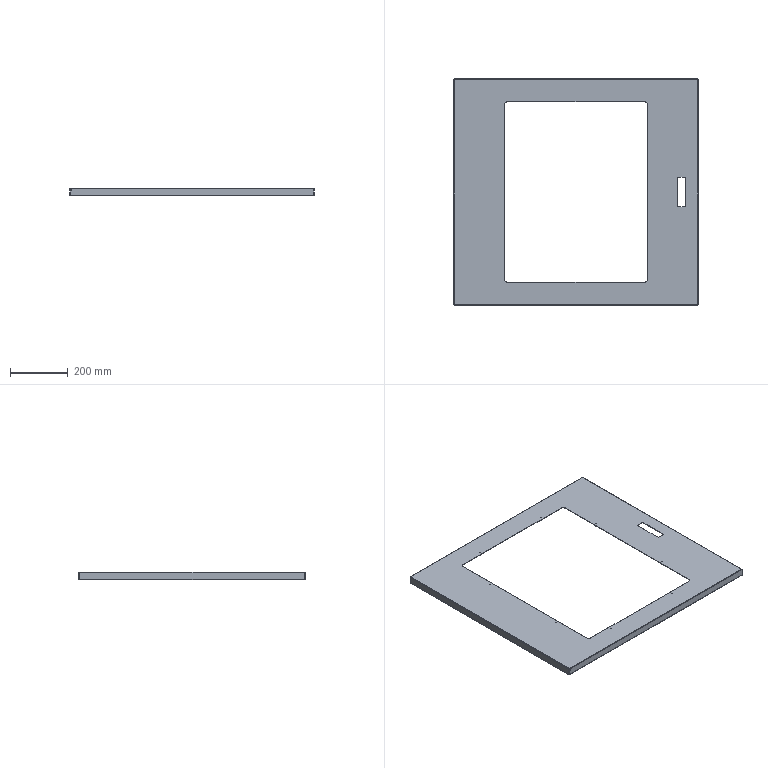Part | SolidWorks | features ICE 4, EdgeFlange 2, MirrorPattern 2, Fillet 1, FlatPattern 1, HoleWzd 1, SMBaseFlange 1, SheetMetal 1 | 1 solid | 110 faces | box 851 x 786 x 26.5 mm | volume 735444 mm3 | plane 54 | cylinder 40 | spline 16 | commonest cylinder face diameters 3 x16 1 x8 4 x8 5 x4 20 x4